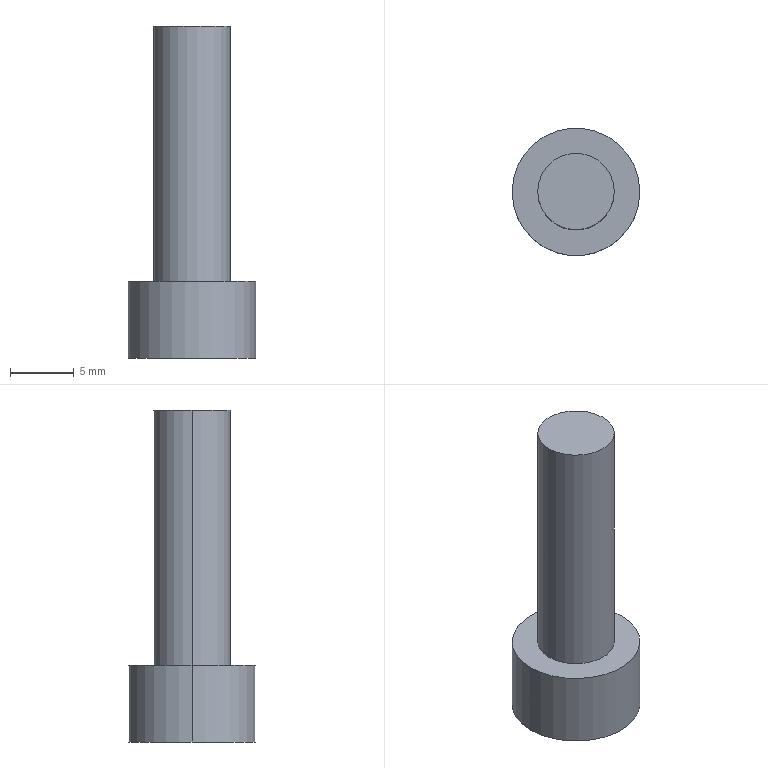Part | STEP file | LG M6_2F | 1 solid | 14 faces | box 10 x 10 x 26 mm | volume 971.253 mm3 | plane 10 | cylinder 4 | commonest cylinder face diameters 6 x2 10 x2
STEP:
#1=CARTESIAN_POINT('',(0.,0.,0.));
#2=DIRECTION('',(0.,0.,1.));
#3=DIRECTION('',(1.,0.,0.));
#4=AXIS2_PLACEMENT_3D('',#1,#2,#3);
#5=CARTESIAN_POINT('',(3.,0.,20.));
#6=VERTEX_POINT('',#5);
#7=CARTESIAN_POINT('',(-3.,0.,20.));
#8=VERTEX_POINT('',#7);
#9=CARTESIAN_POINT('',(0.,0.,20.));
#10=DIRECTION('',(0.,0.,1.));
#11=DIRECTION('',(1.,0.,0.));
#12=AXIS2_PLACEMENT_3D('',#9,#10,#11);
#13=CIRCLE('',#12,3.);
#14=CARTESIAN_POINT('',(0.,0.,20.));
#15=DIRECTION('',(0.,0.,-1.));
#16=DIRECTION('',(-1.,0.,0.));
#17=AXIS2_PLACEMENT_3D('',#14,#15,#16);
#18=CYLINDRICAL_SURFACE('',#17,3.);
#19=CARTESIAN_POINT('',(3.142,0.));
#20=DIRECTION('',(-1.,0.));
#21=VECTOR('',#20,1.);
#22=LINE('',#19,#21);
#23=(GEOMETRIC_REPRESENTATION_CONTEXT(2)PARAMETRIC_REPRESENTATION_CONTEXT()REPRESENTATION_CONTEXT('',''));
#24=DEFINITIONAL_REPRESENTATION('',(#22),#23);
#25=PCURVE('',#18,#24);
#26=CARTESIAN_POINT('',(0.,0.,20.));
#27=DIRECTION('',(0.,0.,1.));
#28=DIRECTION('',(1.,0.,0.));
#29=AXIS2_PLACEMENT_3D('',#26,#27,#28);
#30=PLANE('',#29);
#31=CARTESIAN_POINT('',(0.,0.));
#32=DIRECTION('',(1.,0.));
#33=AXIS2_PLACEMENT_2D('',#31,#32);
#34=CIRCLE('',#33,3.);
#35=(GEOMETRIC_REPRESENTATION_CONTEXT(2)PARAMETRIC_REPRESENTATION_CONTEXT()REPRESENTATION_CONTEXT('',''));
#36=DEFINITIONAL_REPRESENTATION('',(#34),#35);
#37=PCURVE('',#30,#36);
#38=SURFACE_CURVE('',#13,(#25,#37),.PCURVE_S1.);
#39=EDGE_CURVE('',#6,#8,#38,.T.);
#40=ORIENTED_EDGE('',*,*,#39,.F.);
#41=CARTESIAN_POINT('',(3.,0.,0.));
#42=VERTEX_POINT('',#41);
#43=CARTESIAN_POINT('',(3.,0.,20.));
#44=DIRECTION('',(0.,0.,-1.));
#45=VECTOR('',#44,1.);
#46=LINE('',#43,#45);
#47=CARTESIAN_POINT('',(3.142,0.));
#48=DIRECTION('',(0.,1.));
#49=VECTOR('',#48,1.);
#50=LINE('',#47,#49);
#51=(GEOMETRIC_REPRESENTATION_CONTEXT(2)PARAMETRIC_REPRESENTATION_CONTEXT()REPRESENTATION_CONTEXT('',''));
#52=DEFINITIONAL_REPRESENTATION('',(#50),#51);
#53=PCURVE('',#18,#52);
#54=CARTESIAN_POINT('',(0.,0.,20.));
#55=DIRECTION('',(0.,0.,-1.));
#56=DIRECTION('',(-1.,0.,0.));
#57=AXIS2_PLACEMENT_3D('',#54,#55,#56);
#58=CYLINDRICAL_SURFACE('',#57,3.);
#59=CARTESIAN_POINT('',(3.142,0.));
#60=DIRECTION('',(0.,1.));
#61=VECTOR('',#60,1.);
#62=LINE('',#59,#61);
#63=(GEOMETRIC_REPRESENTATION_CONTEXT(2)PARAMETRIC_REPRESENTATION_CONTEXT()REPRESENTATION_CONTEXT('',''));
#64=DEFINITIONAL_REPRESENTATION('',(#62),#63);
#65=PCURVE('',#58,#64);
#66=SURFACE_CURVE('',#46,(#53,#65),.PCURVE_S1.);
#67=EDGE_CURVE('',#6,#42,#66,.T.);
#68=ORIENTED_EDGE('',*,*,#67,.T.);
#69=CARTESIAN_POINT('',(-3.,0.,0.));
#70=VERTEX_POINT('',#69);
#71=CARTESIAN_POINT('',(0.,0.,0.));
#72=DIRECTION('',(0.,0.,1.));
#73=DIRECTION('',(1.,0.,0.));
#74=AXIS2_PLACEMENT_3D('',#71,#72,#73);
#75=CIRCLE('',#74,3.);
#76=CARTESIAN_POINT('',(3.142,20.));
#77=DIRECTION('',(-1.,0.));
#78=VECTOR('',#77,1.);
#79=LINE('',#76,#78);
#80=(GEOMETRIC_REPRESENTATION_CONTEXT(2)PARAMETRIC_REPRESENTATION_CONTEXT()REPRESENTATION_CONTEXT('',''));
#81=DEFINITIONAL_REPRESENTATION('',(#79),#80);
#82=PCURVE('',#18,#81);
#83=CARTESIAN_POINT('',(0.,0.,0.));
#84=DIRECTION('',(0.,0.,1.));
#85=DIRECTION('',(1.,0.,0.));
#86=AXIS2_PLACEMENT_3D('',#83,#84,#85);
#87=PLANE('',#86);
#88=CARTESIAN_POINT('',(0.,0.));
#89=DIRECTION('',(1.,0.));
#90=AXIS2_PLACEMENT_2D('',#88,#89);
#91=CIRCLE('',#90,3.);
#92=(GEOMETRIC_REPRESENTATION_CONTEXT(2)PARAMETRIC_REPRESENTATION_CONTEXT()REPRESENTATION_CONTEXT('',''));
#93=DEFINITIONAL_REPRESENTATION('',(#91),#92);
#94=PCURVE('',#87,#93);
#95=SURFACE_CURVE('',#75,(#82,#94),.PCURVE_S1.);
#96=EDGE_CURVE('',#42,#70,#95,.T.);
#97=ORIENTED_EDGE('',*,*,#96,.T.);
#98=CARTESIAN_POINT('',(-3.,0.,20.));
#99=DIRECTION('',(0.,0.,-1.));
#100=VECTOR('',#99,1.);
#101=LINE('',#98,#100);
#102=CARTESIAN_POINT('',(0.,0.));
#103=DIRECTION('',(0.,1.));
#104=VECTOR('',#103,1.);
#105=LINE('',#102,#104);
#106=(GEOMETRIC_REPRESENTATION_CONTEXT(2)PARAMETRIC_REPRESENTATION_CONTEXT()REPRESENTATION_CONTEXT('',''));
#107=DEFINITIONAL_REPRESENTATION('',(#105),#106);
#108=PCURVE('',#18,#107);
#109=CARTESIAN_POINT('',(6.283,0.));
#110=DIRECTION('',(0.,1.));
#111=VECTOR('',#110,1.);
#112=LINE('',#109,#111);
#113=(GEOMETRIC_REPRESENTATION_CONTEXT(2)PARAMETRIC_REPRESENTATION_CONTEXT()REPRESENTATION_CONTEXT('',''));
#114=DEFINITIONAL_REPRESENTATION('',(#112),#113);
#115=PCURVE('',#58,#114);
#116=SURFACE_CURVE('',#101,(#108,#115),.PCURVE_S1.);
#117=EDGE_CURVE('',#8,#70,#116,.T.);
#118=ORIENTED_EDGE('',*,*,#117,.F.);
#119=EDGE_LOOP('',(#40,#68,#97,#118));
#120=FACE_BOUND('',#119,.T.);
#121=ADVANCED_FACE('',(#120),#18,.T.);
#122=CARTESIAN_POINT('',(5.,0.,-6.));
#123=VERTEX_POINT('',#122);
#124=CARTESIAN_POINT('',(-5.,0.,-6.));
#125=VERTEX_POINT('',#124);
#126=CARTESIAN_POINT('',(0.,0.,-6.));
#127=DIRECTION('',(0.,0.,1.));
#128=DIRECTION('',(1.,0.,0.));
#129=AXIS2_PLACEMENT_3D('',#126,#127,#128);
#130=CIRCLE('',#129,5.);
#131=CARTESIAN_POINT('',(0.,0.,-6.));
#132=DIRECTION('',(0.,0.,1.));
#133=DIRECTION('',(1.,0.,0.));
#134=AXIS2_PLACEMENT_3D('',#131,#132,#133);
#135=CYLINDRICAL_SURFACE('',#134,5.);
#136=CARTESIAN_POINT('',(0.,0.));
#137=DIRECTION('',(1.,0.));
#138=VECTOR('',#137,1.);
#139=LINE('',#136,#138);
#140=(GEOMETRIC_REPRESENTATION_CONTEXT(2)PARAMETRIC_REPRESENTATION_CONTEXT()REPRESENTATION_CONTEXT('',''));
#141=DEFINITIONAL_REPRESENTATION('',(#139),#140);
#142=PCURVE('',#135,#141);
#143=CARTESIAN_POINT('',(0.,0.,-6.));
#144=DIRECTION('',(0.,0.,1.));
#145=DIRECTION('',(1.,0.,0.));
#146=AXIS2_PLACEMENT_3D('',#143,#144,#145);
#147=PLANE('',#146);
#148=CARTESIAN_POINT('',(0.,0.));
#149=DIRECTION('',(1.,0.));
#150=AXIS2_PLACEMENT_2D('',#148,#149);
#151=CIRCLE('',#150,5.);
#152=(GEOMETRIC_REPRESENTATION_CONTEXT(2)PARAMETRIC_REPRESENTATION_CONTEXT()REPRESENTATION_CONTEXT('',''));
#153=DEFINITIONAL_REPRESENTATION('',(#151),#152);
#154=PCURVE('',#147,#153);
#155=SURFACE_CURVE('',#130,(#142,#154),.PCURVE_S1.);
#156=EDGE_CURVE('',#123,#125,#155,.T.);
#157=ORIENTED_EDGE('',*,*,#156,.T.);
#158=CARTESIAN_POINT('',(-5.,0.,0.));
#159=VERTEX_POINT('',#158);
#160=CARTESIAN_POINT('',(-5.,0.,-6.));
#161=DIRECTION('',(0.,0.,1.));
#162=VECTOR('',#161,1.);
#163=LINE('',#160,#162);
#164=CARTESIAN_POINT('',(3.142,0.));
#165=DIRECTION('',(0.,1.));
#166=VECTOR('',#165,1.);
#167=LINE('',#164,#166);
#168=(GEOMETRIC_REPRESENTATION_CONTEXT(2)PARAMETRIC_REPRESENTATION_CONTEXT()REPRESENTATION_CONTEXT('',''));
#169=DEFINITIONAL_REPRESENTATION('',(#167),#168);
#170=PCURVE('',#135,#169);
#171=CARTESIAN_POINT('',(0.,0.,-6.));
#172=DIRECTION('',(0.,0.,1.));
#173=DIRECTION('',(1.,0.,0.));
#174=AXIS2_PLACEMENT_3D('',#171,#172,#173);
#175=CYLINDRICAL_SURFACE('',#174,5.);
#176=CARTESIAN_POINT('',(3.142,0.));
#177=DIRECTION('',(0.,1.));
#178=VECTOR('',#177,1.);
#179=LINE('',#176,#178);
#180=(GEOMETRIC_REPRESENTATION_CONTEXT(2)PARAMETRIC_REPRESENTATION_CONTEXT()REPRESENTATION_CONTEXT('',''));
#181=DEFINITIONAL_REPRESENTATION('',(#179),#180);
#182=PCURVE('',#175,#181);
#183=SURFACE_CURVE('',#163,(#170,#182),.PCURVE_S1.);
#184=EDGE_CURVE('',#125,#159,#183,.T.);
#185=ORIENTED_EDGE('',*,*,#184,.T.);
#186=CARTESIAN_POINT('',(5.,0.,0.));
#187=VERTEX_POINT('',#186);
#188=CARTESIAN_POINT('',(0.,0.,0.));
#189=DIRECTION('',(0.,0.,1.));
#190=DIRECTION('',(1.,0.,0.));
#191=AXIS2_PLACEMENT_3D('',#188,#189,#190);
#192=CIRCLE('',#191,5.);
#193=CARTESIAN_POINT('',(0.,6.));
#194=DIRECTION('',(1.,0.));
#195=VECTOR('',#194,1.);
#196=LINE('',#193,#195);
#197=(GEOMETRIC_REPRESENTATION_CONTEXT(2)PARAMETRIC_REPRESENTATION_CONTEXT()REPRESENTATION_CONTEXT('',''));
#198=DEFINITIONAL_REPRESENTATION('',(#196),#197);
#199=PCURVE('',#135,#198);
#200=CARTESIAN_POINT('',(0.,0.));
#201=DIRECTION('',(1.,0.));
#202=AXIS2_PLACEMENT_2D('',#200,#201);
#203=CIRCLE('',#202,5.);
#204=(GEOMETRIC_REPRESENTATION_CONTEXT(2)PARAMETRIC_REPRESENTATION_CONTEXT()REPRESENTATION_CONTEXT('',''));
#205=DEFINITIONAL_REPRESENTATION('',(#203),#204);
#206=PCURVE('',#87,#205);
#207=SURFACE_CURVE('',#192,(#199,#206),.PCURVE_S1.);
#208=EDGE_CURVE('',#187,#159,#207,.T.);
#209=ORIENTED_EDGE('',*,*,#208,.F.);
#210=CARTESIAN_POINT('',(5.,0.,-6.));
#211=DIRECTION('',(0.,0.,1.));
#212=VECTOR('',#211,1.);
#213=LINE('',#210,#212);
#214=CARTESIAN_POINT('',(0.,0.));
#215=DIRECTION('',(0.,1.));
#216=VECTOR('',#215,1.);
#217=LINE('',#214,#216);
#218=(GEOMETRIC_REPRESENTATION_CONTEXT(2)PARAMETRIC_REPRESENTATION_CONTEXT()REPRESENTATION_CONTEXT('',''));
#219=DEFINITIONAL_REPRESENTATION('',(#217),#218);
#220=PCURVE('',#135,#219);
#221=CARTESIAN_POINT('',(6.283,0.));
#222=DIRECTION('',(0.,1.));
#223=VECTOR('',#222,1.);
#224=LINE('',#221,#223);
#225=(GEOMETRIC_REPRESENTATION_CONTEXT(2)PARAMETRIC_REPRESENTATION_CONTEXT()REPRESENTATION_CONTEXT('',''));
#226=DEFINITIONAL_REPRESENTATION('',(#224),#225);
#227=PCURVE('',#175,#226);
#228=SURFACE_CURVE('',#213,(#220,#227),.PCURVE_S1.);
#229=EDGE_CURVE('',#123,#187,#228,.T.);
#230=ORIENTED_EDGE('',*,*,#229,.F.);
#231=EDGE_LOOP('',(#157,#185,#209,#230));
#232=FACE_BOUND('',#231,.T.);
#233=ADVANCED_FACE('',(#232),#135,.T.);
#234=ORIENTED_EDGE('',*,*,#208,.T.);
#235=CARTESIAN_POINT('',(0.,0.,0.));
#236=DIRECTION('',(0.,0.,1.));
#237=DIRECTION('',(1.,0.,0.));
#238=AXIS2_PLACEMENT_3D('',#235,#236,#237);
#239=CIRCLE('',#238,5.);
#240=CARTESIAN_POINT('',(0.,0.));
#241=DIRECTION('',(1.,0.));
#242=AXIS2_PLACEMENT_2D('',#240,#241);
#243=CIRCLE('',#242,5.);
#244=(GEOMETRIC_REPRESENTATION_CONTEXT(2)PARAMETRIC_REPRESENTATION_CONTEXT()REPRESENTATION_CONTEXT('',''));
#245=DEFINITIONAL_REPRESENTATION('',(#243),#244);
#246=PCURVE('',#87,#245);
#247=CARTESIAN_POINT('',(0.,6.));
#248=DIRECTION('',(1.,0.));
#249=VECTOR('',#248,1.);
#250=LINE('',#247,#249);
#251=(GEOMETRIC_REPRESENTATION_CONTEXT(2)PARAMETRIC_REPRESENTATION_CONTEXT()REPRESENTATION_CONTEXT('',''));
#252=DEFINITIONAL_REPRESENTATION('',(#250),#251);
#253=PCURVE('',#175,#252);
#254=SURFACE_CURVE('',#239,(#246,#253),.PCURVE_S1.);
#255=EDGE_CURVE('',#159,#187,#254,.T.);
#256=ORIENTED_EDGE('',*,*,#255,.T.);
#257=EDGE_LOOP('',(#234,#256));
#258=FACE_BOUND('',#257,.T.);
#259=CARTESIAN_POINT('',(0.,0.,0.));
#260=DIRECTION('',(0.,0.,1.));
#261=DIRECTION('',(1.,0.,0.));
#262=AXIS2_PLACEMENT_3D('',#259,#260,#261);
#263=CIRCLE('',#262,3.);
#264=CARTESIAN_POINT('',(0.,0.));
#265=DIRECTION('',(1.,0.));
#266=AXIS2_PLACEMENT_2D('',#264,#265);
#267=CIRCLE('',#266,3.);
#268=(GEOMETRIC_REPRESENTATION_CONTEXT(2)PARAMETRIC_REPRESENTATION_CONTEXT()REPRESENTATION_CONTEXT('',''));
#269=DEFINITIONAL_REPRESENTATION('',(#267),#268);
#270=PCURVE('',#87,#269);
#271=CARTESIAN_POINT('',(9.425,20.));
#272=DIRECTION('',(-1.,0.));
#273=VECTOR('',#272,1.);
#274=LINE('',#271,#273);
#275=(GEOMETRIC_REPRESENTATION_CONTEXT(2)PARAMETRIC_REPRESENTATION_CONTEXT()REPRESENTATION_CONTEXT('',''));
#276=DEFINITIONAL_REPRESENTATION('',(#274),#275);
#277=PCURVE('',#58,#276);
#278=SURFACE_CURVE('',#263,(#270,#277),.PCURVE_S1.);
#279=EDGE_CURVE('',#70,#42,#278,.T.);
#280=ORIENTED_EDGE('',*,*,#279,.F.);
#281=ORIENTED_EDGE('',*,*,#96,.F.);
#282=EDGE_LOOP('',(#280,#281));
#283=FACE_BOUND('',#282,.T.);
#284=ADVANCED_FACE('',(#258,#283),#87,.T.);
#285=ORIENTED_EDGE('',*,*,#184,.F.);
#286=CARTESIAN_POINT('',(0.,0.,-6.));
#287=DIRECTION('',(0.,0.,1.));
#288=DIRECTION('',(1.,0.,0.));
#289=AXIS2_PLACEMENT_3D('',#286,#287,#288);
#290=CIRCLE('',#289,5.);
#291=CARTESIAN_POINT('',(0.,0.));
#292=DIRECTION('',(1.,0.));
#293=VECTOR('',#292,1.);
#294=LINE('',#291,#293);
#295=(GEOMETRIC_REPRESENTATION_CONTEXT(2)PARAMETRIC_REPRESENTATION_CONTEXT()REPRESENTATION_CONTEXT('',''));
#296=DEFINITIONAL_REPRESENTATION('',(#294),#295);
#297=PCURVE('',#175,#296);
#298=CARTESIAN_POINT('',(0.,0.));
#299=DIRECTION('',(1.,0.));
#300=AXIS2_PLACEMENT_2D('',#298,#299);
#301=CIRCLE('',#300,5.);
#302=(GEOMETRIC_REPRESENTATION_CONTEXT(2)PARAMETRIC_REPRESENTATION_CONTEXT()REPRESENTATION_CONTEXT('',''));
#303=DEFINITIONAL_REPRESENTATION('',(#301),#302);
#304=PCURVE('',#147,#303);
#305=SURFACE_CURVE('',#290,(#297,#304),.PCURVE_S1.);
#306=EDGE_CURVE('',#125,#123,#305,.T.);
#307=ORIENTED_EDGE('',*,*,#306,.T.);
#308=ORIENTED_EDGE('',*,*,#229,.T.);
#309=ORIENTED_EDGE('',*,*,#255,.F.);
#310=EDGE_LOOP('',(#285,#307,#308,#309));
#311=FACE_BOUND('',#310,.T.);
#312=ADVANCED_FACE('',(#311),#175,.T.);
#313=CARTESIAN_POINT('',(-2.898,0.,-6.));
#314=VERTEX_POINT('',#313);
#315=CARTESIAN_POINT('',(-1.449,2.51,-6.));
#316=VERTEX_POINT('',#315);
#317=CARTESIAN_POINT('',(-2.898,0.,-6.));
#318=DIRECTION('',(0.5,0.866,0.));
#319=VECTOR('',#318,1.);
#320=LINE('',#317,#319);
#321=CARTESIAN_POINT('',(-2.898,0.));
#322=DIRECTION('',(0.5,0.866));
#323=VECTOR('',#322,1.);
#324=LINE('',#321,#323);
#325=(GEOMETRIC_REPRESENTATION_CONTEXT(2)PARAMETRIC_REPRESENTATION_CONTEXT()REPRESENTATION_CONTEXT('',''));
#326=DEFINITIONAL_REPRESENTATION('',(#324),#325);
#327=PCURVE('',#147,#326);
#328=CARTESIAN_POINT('',(-2.898,0.,-3.));
#329=DIRECTION('',(-0.866,0.5,0.));
#330=DIRECTION('',(-0.5,-0.866,0.));
#331=AXIS2_PLACEMENT_3D('',#328,#329,#330);
#332=PLANE('',#331);
#333=CARTESIAN_POINT('',(0.,-3.));
#334=DIRECTION('',(-1.,0.));
#335=VECTOR('',#334,1.);
#336=LINE('',#333,#335);
#337=(GEOMETRIC_REPRESENTATION_CONTEXT(2)PARAMETRIC_REPRESENTATION_CONTEXT()REPRESENTATION_CONTEXT('',''));
#338=DEFINITIONAL_REPRESENTATION('',(#336),#337);
#339=PCURVE('',#332,#338);
#340=SURFACE_CURVE('',#320,(#327,#339),.PCURVE_S1.);
#341=EDGE_CURVE('',#314,#316,#340,.T.);
#342=ORIENTED_EDGE('',*,*,#341,.F.);
#343=CARTESIAN_POINT('',(-1.449,-2.51,-6.));
#344=VERTEX_POINT('',#343);
#345=CARTESIAN_POINT('',(-1.449,-2.51,-6.));
#346=DIRECTION('',(-0.5,0.866,0.));
#347=VECTOR('',#346,1.);
#348=LINE('',#345,#347);
#349=CARTESIAN_POINT('',(-1.449,-2.51));
#350=DIRECTION('',(-0.5,0.866));
#351=VECTOR('',#350,1.);
#352=LINE('',#349,#351);
#353=(GEOMETRIC_REPRESENTATION_CONTEXT(2)PARAMETRIC_REPRESENTATION_CONTEXT()REPRESENTATION_CONTEXT('',''));
#354=DEFINITIONAL_REPRESENTATION('',(#352),#353);
#355=PCURVE('',#147,#354);
#356=CARTESIAN_POINT('',(-1.449,-2.51,-3.));
#357=DIRECTION('',(-0.866,-0.5,0.));
#358=DIRECTION('',(0.5,-0.866,0.));
#359=AXIS2_PLACEMENT_3D('',#356,#357,#358);
#360=PLANE('',#359);
#361=CARTESIAN_POINT('',(0.,-3.));
#362=DIRECTION('',(-1.,0.));
#363=VECTOR('',#362,1.);
#364=LINE('',#361,#363);
#365=(GEOMETRIC_REPRESENTATION_CONTEXT(2)PARAMETRIC_REPRESENTATION_CONTEXT()REPRESENTATION_CONTEXT('',''));
#366=DEFINITIONAL_REPRESENTATION('',(#364),#365);
#367=PCURVE('',#360,#366);
#368=SURFACE_CURVE('',#348,(#355,#367),.PCURVE_S1.);
#369=EDGE_CURVE('',#344,#314,#368,.T.);
#370=ORIENTED_EDGE('',*,*,#369,.F.);
#371=CARTESIAN_POINT('',(1.449,-2.51,-6.));
#372=VERTEX_POINT('',#371);
#373=CARTESIAN_POINT('',(1.449,-2.51,-6.));
#374=DIRECTION('',(-1.,0.,0.));
#375=VECTOR('',#374,1.);
#376=LINE('',#373,#375);
#377=CARTESIAN_POINT('',(1.449,-2.51));
#378=DIRECTION('',(-1.,0.));
#379=VECTOR('',#378,1.);
#380=LINE('',#377,#379);
#381=(GEOMETRIC_REPRESENTATION_CONTEXT(2)PARAMETRIC_REPRESENTATION_CONTEXT()REPRESENTATION_CONTEXT('',''));
#382=DEFINITIONAL_REPRESENTATION('',(#380),#381);
#383=PCURVE('',#147,#382);
#384=CARTESIAN_POINT('',(1.449,-2.51,-3.));
#385=DIRECTION('',(0.,-1.,0.));
#386=DIRECTION('',(0.,0.,-1.));
#387=AXIS2_PLACEMENT_3D('',#384,#385,#386);
#388=PLANE('',#387);
#389=CARTESIAN_POINT('',(3.,0.));
#390=DIRECTION('',(0.,-1.));
#391=VECTOR('',#390,1.);
#392=LINE('',#389,#391);
#393=(GEOMETRIC_REPRESENTATION_CONTEXT(2)PARAMETRIC_REPRESENTATION_CONTEXT()REPRESENTATION_CONTEXT('',''));
#394=DEFINITIONAL_REPRESENTATION('',(#392),#393);
#395=PCURVE('',#388,#394);
#396=SURFACE_CURVE('',#376,(#383,#395),.PCURVE_S1.);
#397=EDGE_CURVE('',#372,#344,#396,.T.);
#398=ORIENTED_EDGE('',*,*,#397,.F.);
#399=CARTESIAN_POINT('',(2.898,0.,-6.));
#400=VERTEX_POINT('',#399);
#401=CARTESIAN_POINT('',(2.898,0.,-6.));
#402=DIRECTION('',(-0.5,-0.866,0.));
#403=VECTOR('',#402,1.);
#404=LINE('',#401,#403);
#405=CARTESIAN_POINT('',(2.898,0.));
#406=DIRECTION('',(-0.5,-0.866));
#407=VECTOR('',#406,1.);
#408=LINE('',#405,#407);
#409=(GEOMETRIC_REPRESENTATION_CONTEXT(2)PARAMETRIC_REPRESENTATION_CONTEXT()REPRESENTATION_CONTEXT('',''));
#410=DEFINITIONAL_REPRESENTATION('',(#408),#409);
#411=PCURVE('',#147,#410);
#412=CARTESIAN_POINT('',(2.898,0.,-3.));
#413=DIRECTION('',(0.866,-0.5,0.));
#414=DIRECTION('',(0.5,0.866,0.));
#415=AXIS2_PLACEMENT_3D('',#412,#413,#414);
#416=PLANE('',#415);
#417=CARTESIAN_POINT('',(0.,-3.));
#418=DIRECTION('',(-1.,0.));
#419=VECTOR('',#418,1.);
#420=LINE('',#417,#419);
#421=(GEOMETRIC_REPRESENTATION_CONTEXT(2)PARAMETRIC_REPRESENTATION_CONTEXT()REPRESENTATION_CONTEXT('',''));
#422=DEFINITIONAL_REPRESENTATION('',(#420),#421);
#423=PCURVE('',#416,#422);
#424=SURFACE_CURVE('',#404,(#411,#423),.PCURVE_S1.);
#425=EDGE_CURVE('',#400,#372,#424,.T.);
#426=ORIENTED_EDGE('',*,*,#425,.F.);
#427=CARTESIAN_POINT('',(1.449,2.51,-6.));
#428=VERTEX_POINT('',#427);
#429=CARTESIAN_POINT('',(1.449,2.51,-6.));
#430=DIRECTION('',(0.5,-0.866,0.));
#431=VECTOR('',#430,1.);
#432=LINE('',#429,#431);
#433=CARTESIAN_POINT('',(1.449,2.51));
#434=DIRECTION('',(0.5,-0.866));
#435=VECTOR('',#434,1.);
#436=LINE('',#433,#435);
#437=(GEOMETRIC_REPRESENTATION_CONTEXT(2)PARAMETRIC_REPRESENTATION_CONTEXT()REPRESENTATION_CONTEXT('',''));
#438=DEFINITIONAL_REPRESENTATION('',(#436),#437);
#439=PCURVE('',#147,#438);
#440=CARTESIAN_POINT('',(1.449,2.51,-3.));
#441=DIRECTION('',(0.866,0.5,0.));
#442=DIRECTION('',(-0.5,0.866,0.));
#443=AXIS2_PLACEMENT_3D('',#440,#441,#442);
#444=PLANE('',#443);
#445=CARTESIAN_POINT('',(0.,-3.));
#446=DIRECTION('',(-1.,0.));
#447=VECTOR('',#446,1.);
#448=LINE('',#445,#447);
#449=(GEOMETRIC_REPRESENTATION_CONTEXT(2)PARAMETRIC_REPRESENTATION_CONTEXT()REPRESENTATION_CONTEXT('',''));
#450=DEFINITIONAL_REPRESENTATION('',(#448),#449);
#451=PCURVE('',#444,#450);
#452=SURFACE_CURVE('',#432,(#439,#451),.PCURVE_S1.);
#453=EDGE_CURVE('',#428,#400,#452,.T.);
#454=ORIENTED_EDGE('',*,*,#453,.F.);
#455=CARTESIAN_POINT('',(-1.449,2.51,-6.));
#456=DIRECTION('',(1.,0.,0.));
#457=VECTOR('',#456,1.);
#458=LINE('',#455,#457);
#459=CARTESIAN_POINT('',(-1.449,2.51));
#460=DIRECTION('',(1.,0.));
#461=VECTOR('',#460,1.);
#462=LINE('',#459,#461);
#463=(GEOMETRIC_REPRESENTATION_CONTEXT(2)PARAMETRIC_REPRESENTATION_CONTEXT()REPRESENTATION_CONTEXT('',''));
#464=DEFINITIONAL_REPRESENTATION('',(#462),#463);
#465=PCURVE('',#147,#464);
#466=CARTESIAN_POINT('',(-1.449,2.51,-3.));
#467=DIRECTION('',(0.,1.,0.));
#468=DIRECTION('',(0.,0.,1.));
#469=AXIS2_PLACEMENT_3D('',#466,#467,#468);
#470=PLANE('',#469);
#471=CARTESIAN_POINT('',(-3.,0.));
#472=DIRECTION('',(0.,1.));
#473=VECTOR('',#472,1.);
#474=LINE('',#471,#473);
#475=(GEOMETRIC_REPRESENTATION_CONTEXT(2)PARAMETRIC_REPRESENTATION_CONTEXT()REPRESENTATION_CONTEXT('',''));
#476=DEFINITIONAL_REPRESENTATION('',(#474),#475);
#477=PCURVE('',#470,#476);
#478=SURFACE_CURVE('',#458,(#465,#477),.PCURVE_S1.);
#479=EDGE_CURVE('',#316,#428,#478,.T.);
#480=ORIENTED_EDGE('',*,*,#479,.F.);
#481=EDGE_LOOP('',(#342,#370,#398,#426,#454,#480));
#482=FACE_BOUND('',#481,.T.);
#483=ORIENTED_EDGE('',*,*,#156,.F.);
#484=ORIENTED_EDGE('',*,*,#306,.F.);
#485=EDGE_LOOP('',(#483,#484));
#486=FACE_BOUND('',#485,.T.);
#487=ADVANCED_FACE('',(#482,#486),#147,.F.);
#488=ORIENTED_EDGE('',*,*,#67,.F.);
#489=CARTESIAN_POINT('',(0.,0.,20.));
#490=DIRECTION('',(0.,0.,1.));
#491=DIRECTION('',(1.,0.,0.));
#492=AXIS2_PLACEMENT_3D('',#489,#490,#491);
#493=CIRCLE('',#492,3.);
#494=CARTESIAN_POINT('',(9.425,0.));
#495=DIRECTION('',(-1.,0.));
#496=VECTOR('',#495,1.);
#497=LINE('',#494,#496);
#498=(GEOMETRIC_REPRESENTATION_CONTEXT(2)PARAMETRIC_REPRESENTATION_CONTEXT()REPRESENTATION_CONTEXT('',''));
#499=DEFINITIONAL_REPRESENTATION('',(#497),#498);
#500=PCURVE('',#58,#499);
#501=CARTESIAN_POINT('',(0.,0.));
#502=DIRECTION('',(1.,0.));
#503=AXIS2_PLACEMENT_2D('',#501,#502);
#504=CIRCLE('',#503,3.);
#505=(GEOMETRIC_REPRESENTATION_CONTEXT(2)PARAMETRIC_REPRESENTATION_CONTEXT()REPRESENTATION_CONTEXT('',''));
#506=DEFINITIONAL_REPRESENTATION('',(#504),#505);
#507=PCURVE('',#30,#506);
#508=SURFACE_CURVE('',#493,(#500,#507),.PCURVE_S1.);
#509=EDGE_CURVE('',#8,#6,#508,.T.);
#510=ORIENTED_EDGE('',*,*,#509,.F.);
#511=ORIENTED_EDGE('',*,*,#117,.T.);
#512=ORIENTED_EDGE('',*,*,#279,.T.);
#513=EDGE_LOOP('',(#488,#510,#511,#512));
#514=FACE_BOUND('',#513,.T.);
#515=ADVANCED_FACE('',(#514),#58,.T.);
#516=ORIENTED_EDGE('',*,*,#509,.T.);
#517=ORIENTED_EDGE('',*,*,#39,.T.);
#518=EDGE_LOOP('',(#516,#517));
#519=FACE_BOUND('',#518,.T.);
#520=ADVANCED_FACE('',(#519),#30,.T.);
#521=ORIENTED_EDGE('',*,*,#369,.T.);
#522=CARTESIAN_POINT('',(-2.898,0.,-3.));
#523=VERTEX_POINT('',#522);
#524=CARTESIAN_POINT('',(-2.898,0.,-3.));
#525=DIRECTION('',(0.,0.,-1.));
#526=VECTOR('',#525,1.);
#527=LINE('',#524,#526);
#528=CARTESIAN_POINT('',(-2.898,0.));
#529=DIRECTION('',(0.,-1.));
#530=VECTOR('',#529,1.);
#531=LINE('',#528,#530);
#532=(GEOMETRIC_REPRESENTATION_CONTEXT(2)PARAMETRIC_REPRESENTATION_CONTEXT()REPRESENTATION_CONTEXT('',''));
#533=DEFINITIONAL_REPRESENTATION('',(#531),#532);
#534=PCURVE('',#360,#533);
#535=CARTESIAN_POINT('',(0.,0.));
#536=DIRECTION('',(0.,-1.));
#537=VECTOR('',#536,1.);
#538=LINE('',#535,#537);
#539=(GEOMETRIC_REPRESENTATION_CONTEXT(2)PARAMETRIC_REPRESENTATION_CONTEXT()REPRESENTATION_CONTEXT('',''));
#540=DEFINITIONAL_REPRESENTATION('',(#538),#539);
#541=PCURVE('',#332,#540);
#542=SURFACE_CURVE('',#527,(#534,#541),.PCURVE_S1.);
#543=EDGE_CURVE('',#523,#314,#542,.T.);
#544=ORIENTED_EDGE('',*,*,#543,.F.);
#545=CARTESIAN_POINT('',(-1.449,-2.51,-3.));
#546=VERTEX_POINT('',#545);
#547=CARTESIAN_POINT('',(-1.449,-2.51,-3.));
#548=DIRECTION('',(-0.5,0.866,0.));
#549=VECTOR('',#548,1.);
#550=LINE('',#547,#549);
#551=CARTESIAN_POINT('',(0.,0.));
#552=DIRECTION('',(-1.,0.));
#553=VECTOR('',#552,1.);
#554=LINE('',#551,#553);
#555=(GEOMETRIC_REPRESENTATION_CONTEXT(2)PARAMETRIC_REPRESENTATION_CONTEXT()REPRESENTATION_CONTEXT('',''));
#556=DEFINITIONAL_REPRESENTATION('',(#554),#555);
#557=PCURVE('',#360,#556);
#558=CARTESIAN_POINT('',(0.,0.,-3.));
#559=DIRECTION('',(0.,0.,-1.));
#560=DIRECTION('',(-1.,0.,0.));
#561=AXIS2_PLACEMENT_3D('',#558,#559,#560);
#562=PLANE('',#561);
#563=CARTESIAN_POINT('',(1.449,-2.51));
#564=DIRECTION('',(0.5,0.866));
#565=VECTOR('',#564,1.);
#566=LINE('',#563,#565);
#567=(GEOMETRIC_REPRESENTATION_CONTEXT(2)PARAMETRIC_REPRESENTATION_CONTEXT()REPRESENTATION_CONTEXT('',''));
#568=DEFINITIONAL_REPRESENTATION('',(#566),#567);
#569=PCURVE('',#562,#568);
#570=SURFACE_CURVE('',#550,(#557,#569),.PCURVE_S1.);
#571=EDGE_CURVE('',#546,#523,#570,.T.);
#572=ORIENTED_EDGE('',*,*,#571,.F.);
#573=CARTESIAN_POINT('',(-1.449,-2.51,-3.));
#574=DIRECTION('',(0.,0.,-1.));
#575=VECTOR('',#574,1.);
#576=LINE('',#573,#575);
#577=CARTESIAN_POINT('',(0.,0.));
#578=DIRECTION('',(0.,-1.));
#579=VECTOR('',#578,1.);
#580=LINE('',#577,#579);
#581=(GEOMETRIC_REPRESENTATION_CONTEXT(2)PARAMETRIC_REPRESENTATION_CONTEXT()REPRESENTATION_CONTEXT('',''));
#582=DEFINITIONAL_REPRESENTATION('',(#580),#581);
#583=PCURVE('',#360,#582);
#584=CARTESIAN_POINT('',(0.,-2.898));
#585=DIRECTION('',(1.,0.));
#586=VECTOR('',#585,1.);
#587=LINE('',#584,#586);
#588=(GEOMETRIC_REPRESENTATION_CONTEXT(2)PARAMETRIC_REPRESENTATION_CONTEXT()REPRESENTATION_CONTEXT('',''));
#589=DEFINITIONAL_REPRESENTATION('',(#587),#588);
#590=PCURVE('',#388,#589);
#591=SURFACE_CURVE('',#576,(#583,#590),.PCURVE_S1.);
#592=EDGE_CURVE('',#546,#344,#591,.T.);
#593=ORIENTED_EDGE('',*,*,#592,.T.);
#594=EDGE_LOOP('',(#521,#544,#572,#593));
#595=FACE_BOUND('',#594,.T.);
#596=ADVANCED_FACE('',(#595),#360,.F.);
#597=ORIENTED_EDGE('',*,*,#397,.T.);
#598=ORIENTED_EDGE('',*,*,#592,.F.);
#599=CARTESIAN_POINT('',(1.449,-2.51,-3.));
#600=VERTEX_POINT('',#599);
#601=CARTESIAN_POINT('',(1.449,-2.51,-3.));
#602=DIRECTION('',(-1.,0.,0.));
#603=VECTOR('',#602,1.);
#604=LINE('',#601,#603);
#605=CARTESIAN_POINT('',(0.,0.));
#606=DIRECTION('',(0.,-1.));
#607=VECTOR('',#606,1.);
#608=LINE('',#605,#607);
#609=(GEOMETRIC_REPRESENTATION_CONTEXT(2)PARAMETRIC_REPRESENTATION_CONTEXT()REPRESENTATION_CONTEXT('',''));
#610=DEFINITIONAL_REPRESENTATION('',(#608),#609);
#611=PCURVE('',#388,#610);
#612=CARTESIAN_POINT('',(-1.449,-2.51));
#613=DIRECTION('',(1.,0.));
#614=VECTOR('',#613,1.);
#615=LINE('',#612,#614);
#616=(GEOMETRIC_REPRESENTATION_CONTEXT(2)PARAMETRIC_REPRESENTATION_CONTEXT()REPRESENTATION_CONTEXT('',''));
#617=DEFINITIONAL_REPRESENTATION('',(#615),#616);
#618=PCURVE('',#562,#617);
#619=SURFACE_CURVE('',#604,(#611,#618),.PCURVE_S1.);
#620=EDGE_CURVE('',#600,#546,#619,.T.);
#621=ORIENTED_EDGE('',*,*,#620,.F.);
#622=CARTESIAN_POINT('',(1.449,-2.51,-3.));
#623=DIRECTION('',(0.,0.,-1.));
#624=VECTOR('',#623,1.);
#625=LINE('',#622,#624);
#626=CARTESIAN_POINT('',(0.,0.));
#627=DIRECTION('',(1.,0.));
#628=VECTOR('',#627,1.);
#629=LINE('',#626,#628);
#630=(GEOMETRIC_REPRESENTATION_CONTEXT(2)PARAMETRIC_REPRESENTATION_CONTEXT()REPRESENTATION_CONTEXT('',''));
#631=DEFINITIONAL_REPRESENTATION('',(#629),#630);
#632=PCURVE('',#388,#631);
#633=CARTESIAN_POINT('',(-2.898,0.));
#634=DIRECTION('',(0.,-1.));
#635=VECTOR('',#634,1.);
#636=LINE('',#633,#635);
#637=(GEOMETRIC_REPRESENTATION_CONTEXT(2)PARAMETRIC_REPRESENTATION_CONTEXT()REPRESENTATION_CONTEXT('',''));
#638=DEFINITIONAL_REPRESENTATION('',(#636),#637);
#639=PCURVE('',#416,#638);
#640=SURFACE_CURVE('',#625,(#632,#639),.PCURVE_S1.);
#641=EDGE_CURVE('',#600,#372,#640,.T.);
#642=ORIENTED_EDGE('',*,*,#641,.T.);
#643=EDGE_LOOP('',(#597,#598,#621,#642));
#644=FACE_BOUND('',#643,.T.);
#645=ADVANCED_FACE('',(#644),#388,.F.);
#646=ORIENTED_EDGE('',*,*,#425,.T.);
#647=ORIENTED_EDGE('',*,*,#641,.F.);
#648=CARTESIAN_POINT('',(2.898,0.,-3.));
#649=VERTEX_POINT('',#648);
#650=CARTESIAN_POINT('',(2.898,0.,-3.));
#651=DIRECTION('',(-0.5,-0.866,0.));
#652=VECTOR('',#651,1.);
#653=LINE('',#650,#652);
#654=CARTESIAN_POINT('',(0.,0.));
#655=DIRECTION('',(-1.,0.));
#656=VECTOR('',#655,1.);
#657=LINE('',#654,#656);
#658=(GEOMETRIC_REPRESENTATION_CONTEXT(2)PARAMETRIC_REPRESENTATION_CONTEXT()REPRESENTATION_CONTEXT('',''));
#659=DEFINITIONAL_REPRESENTATION('',(#657),#658);
#660=PCURVE('',#416,#659);
#661=CARTESIAN_POINT('',(-2.898,0.));
#662=DIRECTION('',(0.5,-0.866));
#663=VECTOR('',#662,1.);
#664=LINE('',#661,#663);
#665=(GEOMETRIC_REPRESENTATION_CONTEXT(2)PARAMETRIC_REPRESENTATION_CONTEXT()REPRESENTATION_CONTEXT('',''));
#666=DEFINITIONAL_REPRESENTATION('',(#664),#665);
#667=PCURVE('',#562,#666);
#668=SURFACE_CURVE('',#653,(#660,#667),.PCURVE_S1.);
#669=EDGE_CURVE('',#649,#600,#668,.T.);
#670=ORIENTED_EDGE('',*,*,#669,.F.);
#671=CARTESIAN_POINT('',(2.898,0.,-3.));
#672=DIRECTION('',(0.,0.,-1.));
#673=VECTOR('',#672,1.);
#674=LINE('',#671,#673);
#675=CARTESIAN_POINT('',(0.,0.));
#676=DIRECTION('',(0.,-1.));
#677=VECTOR('',#676,1.);
#678=LINE('',#675,#677);
#679=(GEOMETRIC_REPRESENTATION_CONTEXT(2)PARAMETRIC_REPRESENTATION_CONTEXT()REPRESENTATION_CONTEXT('',''));
#680=DEFINITIONAL_REPRESENTATION('',(#678),#679);
#681=PCURVE('',#416,#680);
#682=CARTESIAN_POINT('',(-2.898,0.));
#683=DIRECTION('',(0.,-1.));
#684=VECTOR('',#683,1.);
#685=LINE('',#682,#684);
#686=(GEOMETRIC_REPRESENTATION_CONTEXT(2)PARAMETRIC_REPRESENTATION_CONTEXT()REPRESENTATION_CONTEXT('',''));
#687=DEFINITIONAL_REPRESENTATION('',(#685),#686);
#688=PCURVE('',#444,#687);
#689=SURFACE_CURVE('',#674,(#681,#688),.PCURVE_S1.);
#690=EDGE_CURVE('',#649,#400,#689,.T.);
#691=ORIENTED_EDGE('',*,*,#690,.T.);
#692=EDGE_LOOP('',(#646,#647,#670,#691));
#693=FACE_BOUND('',#692,.T.);
#694=ADVANCED_FACE('',(#693),#416,.F.);
#695=ORIENTED_EDGE('',*,*,#453,.T.);
#696=ORIENTED_EDGE('',*,*,#690,.F.);
#697=CARTESIAN_POINT('',(1.449,2.51,-3.));
#698=VERTEX_POINT('',#697);
#699=CARTESIAN_POINT('',(1.449,2.51,-3.));
#700=DIRECTION('',(0.5,-0.866,0.));
#701=VECTOR('',#700,1.);
#702=LINE('',#699,#701);
#703=CARTESIAN_POINT('',(0.,0.));
#704=DIRECTION('',(-1.,0.));
#705=VECTOR('',#704,1.);
#706=LINE('',#703,#705);
#707=(GEOMETRIC_REPRESENTATION_CONTEXT(2)PARAMETRIC_REPRESENTATION_CONTEXT()REPRESENTATION_CONTEXT('',''));
#708=DEFINITIONAL_REPRESENTATION('',(#706),#707);
#709=PCURVE('',#444,#708);
#710=CARTESIAN_POINT('',(-1.449,2.51));
#711=DIRECTION('',(-0.5,-0.866));
#712=VECTOR('',#711,1.);
#713=LINE('',#710,#712);
#714=(GEOMETRIC_REPRESENTATION_CONTEXT(2)PARAMETRIC_REPRESENTATION_CONTEXT()REPRESENTATION_CONTEXT('',''));
#715=DEFINITIONAL_REPRESENTATION('',(#713),#714);
#716=PCURVE('',#562,#715);
#717=SURFACE_CURVE('',#702,(#709,#716),.PCURVE_S1.);
#718=EDGE_CURVE('',#698,#649,#717,.T.);
#719=ORIENTED_EDGE('',*,*,#718,.F.);
#720=CARTESIAN_POINT('',(1.449,2.51,-3.));
#721=DIRECTION('',(0.,0.,-1.));
#722=VECTOR('',#721,1.);
#723=LINE('',#720,#722);
#724=CARTESIAN_POINT('',(0.,0.));
#725=DIRECTION('',(0.,-1.));
#726=VECTOR('',#725,1.);
#727=LINE('',#724,#726);
#728=(GEOMETRIC_REPRESENTATION_CONTEXT(2)PARAMETRIC_REPRESENTATION_CONTEXT()REPRESENTATION_CONTEXT('',''));
#729=DEFINITIONAL_REPRESENTATION('',(#727),#728);
#730=PCURVE('',#444,#729);
#731=CARTESIAN_POINT('',(0.,2.898));
#732=DIRECTION('',(-1.,0.));
#733=VECTOR('',#732,1.);
#734=LINE('',#731,#733);
#735=(GEOMETRIC_REPRESENTATION_CONTEXT(2)PARAMETRIC_REPRESENTATION_CONTEXT()REPRESENTATION_CONTEXT('',''));
#736=DEFINITIONAL_REPRESENTATION('',(#734),#735);
#737=PCURVE('',#470,#736);
#738=SURFACE_CURVE('',#723,(#730,#737),.PCURVE_S1.);
#739=EDGE_CURVE('',#698,#428,#738,.T.);
#740=ORIENTED_EDGE('',*,*,#739,.T.);
#741=EDGE_LOOP('',(#695,#696,#719,#740));
#742=FACE_BOUND('',#741,.T.);
#743=ADVANCED_FACE('',(#742),#444,.F.);
#744=ORIENTED_EDGE('',*,*,#479,.T.);
#745=ORIENTED_EDGE('',*,*,#739,.F.);
#746=CARTESIAN_POINT('',(-1.449,2.51,-3.));
#747=VERTEX_POINT('',#746);
#748=CARTESIAN_POINT('',(-1.449,2.51,-3.));
#749=DIRECTION('',(1.,0.,0.));
#750=VECTOR('',#749,1.);
#751=LINE('',#748,#750);
#752=CARTESIAN_POINT('',(0.,0.));
#753=DIRECTION('',(0.,1.));
#754=VECTOR('',#753,1.);
#755=LINE('',#752,#754);
#756=(GEOMETRIC_REPRESENTATION_CONTEXT(2)PARAMETRIC_REPRESENTATION_CONTEXT()REPRESENTATION_CONTEXT('',''));
#757=DEFINITIONAL_REPRESENTATION('',(#755),#756);
#758=PCURVE('',#470,#757);
#759=CARTESIAN_POINT('',(1.449,2.51));
#760=DIRECTION('',(-1.,0.));
#761=VECTOR('',#760,1.);
#762=LINE('',#759,#761);
#763=(GEOMETRIC_REPRESENTATION_CONTEXT(2)PARAMETRIC_REPRESENTATION_CONTEXT()REPRESENTATION_CONTEXT('',''));
#764=DEFINITIONAL_REPRESENTATION('',(#762),#763);
#765=PCURVE('',#562,#764);
#766=SURFACE_CURVE('',#751,(#758,#765),.PCURVE_S1.);
#767=EDGE_CURVE('',#747,#698,#766,.T.);
#768=ORIENTED_EDGE('',*,*,#767,.F.);
#769=CARTESIAN_POINT('',(-1.449,2.51,-3.));
#770=DIRECTION('',(0.,0.,-1.));
#771=VECTOR('',#770,1.);
#772=LINE('',#769,#771);
#773=CARTESIAN_POINT('',(0.,0.));
#774=DIRECTION('',(-1.,0.));
#775=VECTOR('',#774,1.);
#776=LINE('',#773,#775);
#777=(GEOMETRIC_REPRESENTATION_CONTEXT(2)PARAMETRIC_REPRESENTATION_CONTEXT()REPRESENTATION_CONTEXT('',''));
#778=DEFINITIONAL_REPRESENTATION('',(#776),#777);
#779=PCURVE('',#470,#778);
#780=CARTESIAN_POINT('',(-2.898,0.));
#781=DIRECTION('',(0.,-1.));
#782=VECTOR('',#781,1.);
#783=LINE('',#780,#782);
#784=(GEOMETRIC_REPRESENTATION_CONTEXT(2)PARAMETRIC_REPRESENTATION_CONTEXT()REPRESENTATION_CONTEXT('',''));
#785=DEFINITIONAL_REPRESENTATION('',(#783),#784);
#786=PCURVE('',#332,#785);
#787=SURFACE_CURVE('',#772,(#779,#786),.PCURVE_S1.);
#788=EDGE_CURVE('',#747,#316,#787,.T.);
#789=ORIENTED_EDGE('',*,*,#788,.T.);
#790=EDGE_LOOP('',(#744,#745,#768,#789));
#791=FACE_BOUND('',#790,.T.);
#792=ADVANCED_FACE('',(#791),#470,.F.);
#793=ORIENTED_EDGE('',*,*,#341,.T.);
#794=ORIENTED_EDGE('',*,*,#788,.F.);
#795=CARTESIAN_POINT('',(-2.898,0.,-3.));
#796=DIRECTION('',(0.5,0.866,0.));
#797=VECTOR('',#796,1.);
#798=LINE('',#795,#797);
#799=CARTESIAN_POINT('',(0.,0.));
#800=DIRECTION('',(-1.,0.));
#801=VECTOR('',#800,1.);
#802=LINE('',#799,#801);
#803=(GEOMETRIC_REPRESENTATION_CONTEXT(2)PARAMETRIC_REPRESENTATION_CONTEXT()REPRESENTATION_CONTEXT('',''));
#804=DEFINITIONAL_REPRESENTATION('',(#802),#803);
#805=PCURVE('',#332,#804);
#806=CARTESIAN_POINT('',(2.898,0.));
#807=DIRECTION('',(-0.5,0.866));
#808=VECTOR('',#807,1.);
#809=LINE('',#806,#808);
#810=(GEOMETRIC_REPRESENTATION_CONTEXT(2)PARAMETRIC_REPRESENTATION_CONTEXT()REPRESENTATION_CONTEXT('',''));
#811=DEFINITIONAL_REPRESENTATION('',(#809),#810);
#812=PCURVE('',#562,#811);
#813=SURFACE_CURVE('',#798,(#805,#812),.PCURVE_S1.);
#814=EDGE_CURVE('',#523,#747,#813,.T.);
#815=ORIENTED_EDGE('',*,*,#814,.F.);
#816=ORIENTED_EDGE('',*,*,#543,.T.);
#817=EDGE_LOOP('',(#793,#794,#815,#816));
#818=FACE_BOUND('',#817,.T.);
#819=ADVANCED_FACE('',(#818),#332,.F.);
#820=ORIENTED_EDGE('',*,*,#571,.T.);
#821=ORIENTED_EDGE('',*,*,#814,.T.);
#822=ORIENTED_EDGE('',*,*,#767,.T.);
#823=ORIENTED_EDGE('',*,*,#718,.T.);
#824=ORIENTED_EDGE('',*,*,#669,.T.);
#825=ORIENTED_EDGE('',*,*,#620,.T.);
#826=EDGE_LOOP('',(#820,#821,#822,#823,#824,#825));
#827=FACE_BOUND('',#826,.T.);
#828=ADVANCED_FACE('',(#827),#562,.T.);
#829=CLOSED_SHELL('',(#121,#233,#284,#312,#487,#515,#520,#596,#645,#694,#743,#792,#819,#828));
#830=MANIFOLD_SOLID_BREP('',#829);
#831=(LENGTH_UNIT()NAMED_UNIT(*)SI_UNIT(.MILLI.,.METRE.));
#832=UNCERTAINTY_MEASURE_WITH_UNIT(LENGTH_MEASURE(0.0000001),#831,'','');
#833=(NAMED_UNIT(*)PLANE_ANGLE_UNIT()SI_UNIT($,.RADIAN.));
#834=(NAMED_UNIT(*)SI_UNIT($,.STERADIAN.)SOLID_ANGLE_UNIT());
#835=(GEOMETRIC_REPRESENTATION_CONTEXT(3)GLOBAL_UNCERTAINTY_ASSIGNED_CONTEXT((#832))GLOBAL_UNIT_ASSIGNED_CONTEXT((#831,#833,#834))REPRESENTATION_CONTEXT('',''));
#836=ADVANCED_BREP_SHAPE_REPRESENTATION('',(#4,#830),#835);